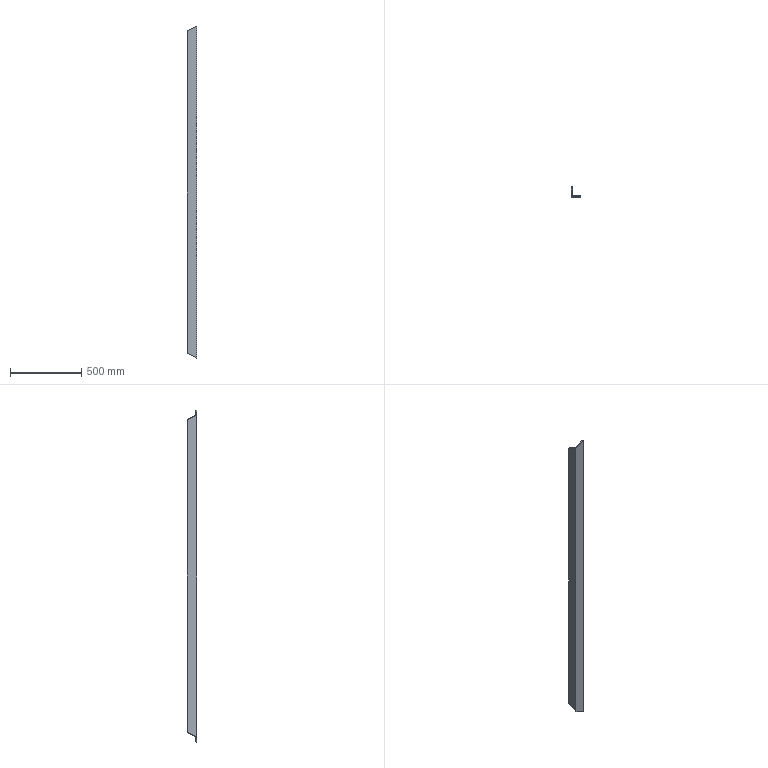Part | SolidWorks | features Extrusion 1, ICE 1 | 1 solid | 11 faces | box 70 x 70 x 2334 mm | volume 2413861 mm3 | plane 8 | cylinder 3 | commonest cylinder face diameters 6 x2 16 x1
STEP:
#1=CARTESIAN_POINT('',(5.,70.,2267.159));
#2=VERTEX_POINT('',#1);
#3=CARTESIAN_POINT('',(0.,70.,2264.683));
#4=VERTEX_POINT('',#3);
#5=CARTESIAN_POINT('',(31.579,70.,2280.318));
#6=DIRECTION('',(-0.8962,0.,-0.4437));
#7=VECTOR('',#6,1000.);
#8=LINE('',#5,#7);
#9=EDGE_CURVE('',#2,#4,#8,.T.);
#10=ORIENTED_EDGE('',*,*,#9,.F.);
#11=CARTESIAN_POINT('',(5.,70.,66.841));
#12=VERTEX_POINT('',#11);
#13=CARTESIAN_POINT('',(5.,70.,2334.));
#14=DIRECTION('',(0.,0.,-1.));
#15=VECTOR('',#14,1000.);
#16=LINE('',#13,#15);
#17=EDGE_CURVE('',#2,#12,#16,.T.);
#18=ORIENTED_EDGE('',*,*,#17,.T.);
#19=CARTESIAN_POINT('',(0.,70.,69.317));
#20=VERTEX_POINT('',#19);
#21=CARTESIAN_POINT('',(-896.516,70.,513.202));
#22=DIRECTION('',(0.8962,0.,-0.4437));
#23=VECTOR('',#22,1000.);
#24=LINE('',#21,#23);
#25=EDGE_CURVE('',#20,#12,#24,.T.);
#26=ORIENTED_EDGE('',*,*,#25,.F.);
#27=CARTESIAN_POINT('',(0.,70.,2334.));
#28=DIRECTION('',(0.,0.,-1.));
#29=VECTOR('',#28,1000.);
#30=LINE('',#27,#29);
#31=EDGE_CURVE('',#4,#20,#30,.T.);
#32=ORIENTED_EDGE('',*,*,#31,.F.);
#33=EDGE_LOOP('',(#10,#18,#26,#32));
#34=FACE_OUTER_BOUND('',#33,.T.);
#35=CARTESIAN_POINT('',(5.,70.,2334.));
#36=DIRECTION('',(0.,-1.,0.));
#37=DIRECTION('',(0.,0.,-1.));
#38=AXIS2_PLACEMENT_3D('',#35,#36,#37);
#39=PLANE('',#38);
#40=ADVANCED_FACE('',(#34),#39,.F.);
#41=CARTESIAN_POINT('',(0.,0.,2299.341));
#42=VERTEX_POINT('',#41);
#43=CARTESIAN_POINT('',(0.,42.437,2278.33));
#44=DIRECTION('',(0.,-0.8962,0.4437));
#45=VECTOR('',#44,1000.);
#46=LINE('',#43,#45);
#47=EDGE_CURVE('',#4,#42,#46,.T.);
#48=ORIENTED_EDGE('',*,*,#47,.F.);
#49=ORIENTED_EDGE('',*,*,#31,.T.);
#50=CARTESIAN_POINT('',(0.,0.,34.659));
#51=VERTEX_POINT('',#50);
#52=CARTESIAN_POINT('',(0.,970.532,515.19));
#53=DIRECTION('',(0.,0.8962,0.4437));
#54=VECTOR('',#53,1000.);
#55=LINE('',#52,#54);
#56=EDGE_CURVE('',#51,#20,#55,.T.);
#57=ORIENTED_EDGE('',*,*,#56,.F.);
#58=CARTESIAN_POINT('',(0.,0.,2334.));
#59=DIRECTION('',(0.,0.,-1.));
#60=VECTOR('',#59,1000.);
#61=LINE('',#58,#60);
#62=EDGE_CURVE('',#42,#51,#61,.T.);
#63=ORIENTED_EDGE('',*,*,#62,.F.);
#64=EDGE_LOOP('',(#48,#49,#57,#63));
#65=FACE_OUTER_BOUND('',#64,.T.);
#66=CARTESIAN_POINT('',(0.,70.,2334.));
#67=DIRECTION('',(1.,0.,0.));
#68=DIRECTION('',(0.,0.,-1.));
#69=AXIS2_PLACEMENT_3D('',#66,#67,#68);
#70=PLANE('',#69);
#71=ADVANCED_FACE('',(#65),#70,.F.);
#72=CARTESIAN_POINT('',(70.,0.,2334.));
#73=VERTEX_POINT('',#72);
#74=CARTESIAN_POINT('',(13.782,0.,2306.165));
#75=DIRECTION('',(0.8962,0.,0.4437));
#76=VECTOR('',#75,1000.);
#77=LINE('',#74,#76);
#78=EDGE_CURVE('',#42,#73,#77,.T.);
#79=ORIENTED_EDGE('',*,*,#78,.F.);
#80=ORIENTED_EDGE('',*,*,#62,.T.);
#81=CARTESIAN_POINT('',(70.,0.,0.));
#82=VERTEX_POINT('',#81);
#83=CARTESIAN_POINT('',(-914.314,0.,487.355));
#84=DIRECTION('',(-0.8962,0.,0.4437));
#85=VECTOR('',#84,1000.);
#86=LINE('',#83,#85);
#87=EDGE_CURVE('',#82,#51,#86,.T.);
#88=ORIENTED_EDGE('',*,*,#87,.F.);
#89=CARTESIAN_POINT('',(70.,0.,2334.));
#90=DIRECTION('',(0.,0.,-1.));
#91=VECTOR('',#90,1000.);
#92=LINE('',#89,#91);
#93=EDGE_CURVE('',#73,#82,#92,.T.);
#94=ORIENTED_EDGE('',*,*,#93,.F.);
#95=EDGE_LOOP('',(#79,#80,#88,#94));
#96=FACE_OUTER_BOUND('',#95,.T.);
#97=CARTESIAN_POINT('',(0.,0.,2334.));
#98=DIRECTION('',(0.,1.,0.));
#99=DIRECTION('',(0.,0.,1.));
#100=AXIS2_PLACEMENT_3D('',#97,#98,#99);
#101=PLANE('',#100);
#102=ADVANCED_FACE('',(#96),#101,.F.);
#103=CARTESIAN_POINT('',(70.,5.,2331.524));
#104=VERTEX_POINT('',#103);
#105=CARTESIAN_POINT('',(70.,0.,2334.));
#106=DIRECTION('',(0.,0.8962,-0.4437));
#107=VECTOR('',#106,1000.);
#108=LINE('',#105,#107);
#109=EDGE_CURVE('',#73,#104,#108,.T.);
#110=ORIENTED_EDGE('',*,*,#109,.F.);
#111=ORIENTED_EDGE('',*,*,#93,.T.);
#112=CARTESIAN_POINT('',(70.,5.,2.476));
#113=VERTEX_POINT('',#112);
#114=CARTESIAN_POINT('',(70.,928.095,459.52));
#115=DIRECTION('',(0.,-0.8962,-0.4437));
#116=VECTOR('',#115,1000.);
#117=LINE('',#114,#116);
#118=EDGE_CURVE('',#113,#82,#117,.T.);
#119=ORIENTED_EDGE('',*,*,#118,.F.);
#120=CARTESIAN_POINT('',(70.,5.,2334.));
#121=DIRECTION('',(0.,0.,-1.));
#122=VECTOR('',#121,1000.);
#123=LINE('',#120,#122);
#124=EDGE_CURVE('',#104,#113,#123,.T.);
#125=ORIENTED_EDGE('',*,*,#124,.F.);
#126=EDGE_LOOP('',(#110,#111,#119,#125));
#127=FACE_OUTER_BOUND('',#126,.T.);
#128=CARTESIAN_POINT('',(70.,0.,2334.));
#129=DIRECTION('',(-1.,0.,0.));
#130=DIRECTION('',(0.,0.,1.));
#131=AXIS2_PLACEMENT_3D('',#128,#129,#130);
#132=PLANE('',#131);
#133=ADVANCED_FACE('',(#127),#132,.F.);
#134=CARTESIAN_POINT('',(67.,8.,2328.554));
#135=VERTEX_POINT('',#134);
#136=CARTESIAN_POINT('',(70.,5.,2331.524));
#137=CARTESIAN_POINT('',(70.,6.757,2330.654));
#138=CARTESIAN_POINT('',(68.757,8.,2329.424));
#139=CARTESIAN_POINT('',(67.,8.,2328.554));
#140=(BOUNDED_CURVE()B_SPLINE_CURVE(3,(#136,#137,#138,#139),.UNSPECIFIED.,.F.,.F.)B_SPLINE_CURVE_WITH_KNOTS((4,4),(3.927,5.498),.UNSPECIFIED.)CURVE()GEOMETRIC_REPRESENTATION_ITEM()RATIONAL_B_SPLINE_CURVE((1.,0.8047,0.8047,1.))REPRESENTATION_ITEM(''));
#141=EDGE_CURVE('',#104,#135,#140,.T.);
#142=ORIENTED_EDGE('',*,*,#141,.F.);
#143=ORIENTED_EDGE('',*,*,#124,.T.);
#144=CARTESIAN_POINT('',(67.,8.,5.446));
#145=VERTEX_POINT('',#144);
#146=CARTESIAN_POINT('',(67.,8.,5.446));
#147=CARTESIAN_POINT('',(68.757,8.,4.576));
#148=CARTESIAN_POINT('',(70.,6.757,3.346));
#149=CARTESIAN_POINT('',(70.,5.,2.476));
#150=(BOUNDED_CURVE()B_SPLINE_CURVE(3,(#146,#147,#148,#149),.UNSPECIFIED.,.F.,.F.)B_SPLINE_CURVE_WITH_KNOTS((4,4),(3.927,5.498),.UNSPECIFIED.)CURVE()GEOMETRIC_REPRESENTATION_ITEM()RATIONAL_B_SPLINE_CURVE((1.,0.8047,0.8047,1.))REPRESENTATION_ITEM(''));
#151=EDGE_CURVE('',#145,#113,#150,.T.);
#152=ORIENTED_EDGE('',*,*,#151,.F.);
#153=CARTESIAN_POINT('',(67.,8.,2334.));
#154=DIRECTION('',(0.,0.,-1.));
#155=VECTOR('',#154,1000.);
#156=LINE('',#153,#155);
#157=EDGE_CURVE('',#135,#145,#156,.T.);
#158=ORIENTED_EDGE('',*,*,#157,.F.);
#159=EDGE_LOOP('',(#142,#143,#152,#158));
#160=FACE_OUTER_BOUND('',#159,.T.);
#161=CARTESIAN_POINT('',(67.,5.,2334.));
#162=DIRECTION('',(0.,0.,-1.));
#163=DIRECTION('',(-1.,0.,0.));
#164=AXIS2_PLACEMENT_3D('',#161,#162,#163);
#165=CYLINDRICAL_SURFACE('',#164,3.);
#166=ADVANCED_FACE('',(#160),#165,.T.);
#167=CARTESIAN_POINT('',(16.,8.,2303.302));
#168=VERTEX_POINT('',#167);
#169=CARTESIAN_POINT('',(69.166,8.,2329.626));
#170=DIRECTION('',(-0.8962,0.,-0.4437));
#171=VECTOR('',#170,1000.);
#172=LINE('',#169,#171);
#173=EDGE_CURVE('',#135,#168,#172,.T.);
#174=ORIENTED_EDGE('',*,*,#173,.F.);
#175=ORIENTED_EDGE('',*,*,#157,.T.);
#176=CARTESIAN_POINT('',(16.,8.,30.698));
#177=VERTEX_POINT('',#176);
#178=CARTESIAN_POINT('',(-858.93,8.,463.894));
#179=DIRECTION('',(0.8962,0.,-0.4437));
#180=VECTOR('',#179,1000.);
#181=LINE('',#178,#180);
#182=EDGE_CURVE('',#177,#145,#181,.T.);
#183=ORIENTED_EDGE('',*,*,#182,.F.);
#184=CARTESIAN_POINT('',(16.,8.,2334.));
#185=DIRECTION('',(0.,0.,-1.));
#186=VECTOR('',#185,1000.);
#187=LINE('',#184,#186);
#188=EDGE_CURVE('',#168,#177,#187,.T.);
#189=ORIENTED_EDGE('',*,*,#188,.F.);
#190=EDGE_LOOP('',(#174,#175,#183,#189));
#191=FACE_OUTER_BOUND('',#190,.T.);
#192=CARTESIAN_POINT('',(67.,8.,2334.));
#193=DIRECTION('',(0.,-1.,0.));
#194=DIRECTION('',(1.,0.,0.));
#195=AXIS2_PLACEMENT_3D('',#192,#193,#194);
#196=PLANE('',#195);
#197=ADVANCED_FACE('',(#191),#196,.F.);
#198=CARTESIAN_POINT('',(8.,16.,2295.381));
#199=VERTEX_POINT('',#198);
#200=CARTESIAN_POINT('',(16.,8.,2303.302));
#201=CARTESIAN_POINT('',(11.314,8.,2300.982));
#202=CARTESIAN_POINT('',(8.,11.314,2297.701));
#203=CARTESIAN_POINT('',(8.,16.,2295.381));
#204=(BOUNDED_CURVE()B_SPLINE_CURVE(3,(#200,#201,#202,#203),.UNSPECIFIED.,.F.,.F.)B_SPLINE_CURVE_WITH_KNOTS((4,4),(3.927,5.498),.UNSPECIFIED.)CURVE()GEOMETRIC_REPRESENTATION_ITEM()RATIONAL_B_SPLINE_CURVE((1.,0.8047,0.8047,1.))REPRESENTATION_ITEM(''));
#205=EDGE_CURVE('',#168,#199,#204,.T.);
#206=ORIENTED_EDGE('',*,*,#205,.F.);
#207=ORIENTED_EDGE('',*,*,#188,.T.);
#208=CARTESIAN_POINT('',(8.,16.,38.619));
#209=VERTEX_POINT('',#208);
#210=CARTESIAN_POINT('',(8.,16.,38.619));
#211=CARTESIAN_POINT('',(8.,11.314,36.299));
#212=CARTESIAN_POINT('',(11.314,8.,33.018));
#213=CARTESIAN_POINT('',(16.,8.,30.698));
#214=(BOUNDED_CURVE()B_SPLINE_CURVE(3,(#210,#211,#212,#213),.UNSPECIFIED.,.F.,.F.)B_SPLINE_CURVE_WITH_KNOTS((4,4),(3.927,5.498),.UNSPECIFIED.)CURVE()GEOMETRIC_REPRESENTATION_ITEM()RATIONAL_B_SPLINE_CURVE((1.,0.8047,0.8047,1.))REPRESENTATION_ITEM(''));
#215=EDGE_CURVE('',#209,#177,#214,.T.);
#216=ORIENTED_EDGE('',*,*,#215,.F.);
#217=CARTESIAN_POINT('',(8.,16.,2334.));
#218=DIRECTION('',(0.,0.,-1.));
#219=VECTOR('',#218,1000.);
#220=LINE('',#217,#219);
#221=EDGE_CURVE('',#199,#209,#220,.T.);
#222=ORIENTED_EDGE('',*,*,#221,.F.);
#223=EDGE_LOOP('',(#206,#207,#216,#222));
#224=FACE_OUTER_BOUND('',#223,.T.);
#225=CARTESIAN_POINT('',(16.,16.,2334.));
#226=DIRECTION('',(0.,0.,-1.));
#227=DIRECTION('',(-1.,0.,0.));
#228=AXIS2_PLACEMENT_3D('',#225,#226,#227);
#229=CYLINDRICAL_SURFACE('',#228,8.);
#230=ADVANCED_FACE('',(#224),#229,.F.);
#231=CARTESIAN_POINT('',(8.,67.,2270.129));
#232=VERTEX_POINT('',#231);
#233=CARTESIAN_POINT('',(8.,0.6433,2302.984));
#234=DIRECTION('',(0.,0.8962,-0.4437));
#235=VECTOR('',#234,1000.);
#236=LINE('',#233,#235);
#237=EDGE_CURVE('',#199,#232,#236,.T.);
#238=ORIENTED_EDGE('',*,*,#237,.F.);
#239=ORIENTED_EDGE('',*,*,#221,.T.);
#240=CARTESIAN_POINT('',(8.,67.,63.871));
#241=VERTEX_POINT('',#240);
#242=CARTESIAN_POINT('',(8.,928.739,490.536));
#243=DIRECTION('',(0.,-0.8962,-0.4437));
#244=VECTOR('',#243,1000.);
#245=LINE('',#242,#244);
#246=EDGE_CURVE('',#241,#209,#245,.T.);
#247=ORIENTED_EDGE('',*,*,#246,.F.);
#248=CARTESIAN_POINT('',(8.,67.,2334.));
#249=DIRECTION('',(0.,0.,-1.));
#250=VECTOR('',#249,1000.);
#251=LINE('',#248,#250);
#252=EDGE_CURVE('',#232,#241,#251,.T.);
#253=ORIENTED_EDGE('',*,*,#252,.F.);
#254=EDGE_LOOP('',(#238,#239,#247,#253));
#255=FACE_OUTER_BOUND('',#254,.T.);
#256=CARTESIAN_POINT('',(8.,16.,2334.));
#257=DIRECTION('',(-1.,0.,0.));
#258=DIRECTION('',(0.,-1.,0.));
#259=AXIS2_PLACEMENT_3D('',#256,#257,#258);
#260=PLANE('',#259);
#261=ADVANCED_FACE('',(#255),#260,.F.);
#262=CARTESIAN_POINT('',(8.,67.,2270.129));
#263=CARTESIAN_POINT('',(8.,68.757,2269.259));
#264=CARTESIAN_POINT('',(6.757,70.,2268.029));
#265=CARTESIAN_POINT('',(5.,70.,2267.159));
#266=(BOUNDED_CURVE()B_SPLINE_CURVE(3,(#262,#263,#264,#265),.UNSPECIFIED.,.F.,.F.)B_SPLINE_CURVE_WITH_KNOTS((4,4),(3.927,5.498),.UNSPECIFIED.)CURVE()GEOMETRIC_REPRESENTATION_ITEM()RATIONAL_B_SPLINE_CURVE((1.,0.8047,0.8047,1.))REPRESENTATION_ITEM(''));
#267=EDGE_CURVE('',#232,#2,#266,.T.);
#268=ORIENTED_EDGE('',*,*,#267,.F.);
#269=ORIENTED_EDGE('',*,*,#252,.T.);
#270=CARTESIAN_POINT('',(5.,70.,66.841));
#271=CARTESIAN_POINT('',(6.757,70.,65.971));
#272=CARTESIAN_POINT('',(8.,68.757,64.741));
#273=CARTESIAN_POINT('',(8.,67.,63.871));
#274=(BOUNDED_CURVE()B_SPLINE_CURVE(3,(#270,#271,#272,#273),.UNSPECIFIED.,.F.,.F.)B_SPLINE_CURVE_WITH_KNOTS((4,4),(3.927,5.498),.UNSPECIFIED.)CURVE()GEOMETRIC_REPRESENTATION_ITEM()RATIONAL_B_SPLINE_CURVE((1.,0.8047,0.8047,1.))REPRESENTATION_ITEM(''));
#275=EDGE_CURVE('',#12,#241,#274,.T.);
#276=ORIENTED_EDGE('',*,*,#275,.F.);
#277=ORIENTED_EDGE('',*,*,#17,.F.);
#278=EDGE_LOOP('',(#268,#269,#276,#277));
#279=FACE_OUTER_BOUND('',#278,.T.);
#280=CARTESIAN_POINT('',(5.,67.,2334.));
#281=DIRECTION('',(0.,0.,-1.));
#282=DIRECTION('',(-1.,0.,0.));
#283=AXIS2_PLACEMENT_3D('',#280,#281,#282);
#284=CYLINDRICAL_SURFACE('',#283,3.);
#285=ADVANCED_FACE('',(#279),#284,.T.);
#286=ORIENTED_EDGE('',*,*,#25,.T.);
#287=ORIENTED_EDGE('',*,*,#275,.T.);
#288=ORIENTED_EDGE('',*,*,#246,.T.);
#289=ORIENTED_EDGE('',*,*,#215,.T.);
#290=ORIENTED_EDGE('',*,*,#182,.T.);
#291=ORIENTED_EDGE('',*,*,#151,.T.);
#292=ORIENTED_EDGE('',*,*,#118,.T.);
#293=ORIENTED_EDGE('',*,*,#87,.T.);
#294=ORIENTED_EDGE('',*,*,#56,.T.);
#295=EDGE_LOOP('',(#286,#287,#288,#289,#290,#291,#292,#293,#294));
#296=FACE_OUTER_BOUND('',#295,.T.);
#297=CARTESIAN_POINT('',(105.,35.,0.));
#298=DIRECTION('',(-0.4056,0.4056,-0.8192));
#299=DIRECTION('',(0.,0.8962,0.4437));
#300=AXIS2_PLACEMENT_3D('',#297,#298,#299);
#301=PLANE('',#300);
#302=ADVANCED_FACE('',(#296),#301,.T.);
#303=ORIENTED_EDGE('',*,*,#9,.T.);
#304=ORIENTED_EDGE('',*,*,#47,.T.);
#305=ORIENTED_EDGE('',*,*,#78,.T.);
#306=ORIENTED_EDGE('',*,*,#109,.T.);
#307=ORIENTED_EDGE('',*,*,#141,.T.);
#308=ORIENTED_EDGE('',*,*,#173,.T.);
#309=ORIENTED_EDGE('',*,*,#205,.T.);
#310=ORIENTED_EDGE('',*,*,#237,.T.);
#311=ORIENTED_EDGE('',*,*,#267,.T.);
#312=EDGE_LOOP('',(#303,#304,#305,#306,#307,#308,#309,#310,#311));
#313=FACE_OUTER_BOUND('',#312,.T.);
#314=CARTESIAN_POINT('',(35.,105.,2264.683));
#315=DIRECTION('',(-0.4056,0.4056,0.8192));
#316=DIRECTION('',(0.,-0.8962,0.4437));
#317=AXIS2_PLACEMENT_3D('',#314,#315,#316);
#318=PLANE('',#317);
#319=ADVANCED_FACE('',(#313),#318,.T.);
#320=CLOSED_SHELL('',(#40,#71,#102,#133,#166,#197,#230,#261,#285,#302,#319));
#321=MANIFOLD_SOLID_BREP('',#320);
#322=CARTESIAN_POINT('',(0.,0.,0.));
#323=DIRECTION('',(0.,0.,1.));
#324=DIRECTION('',(1.,0.,0.));
#325=AXIS2_PLACEMENT_3D('',#322,#323,#324);
#326=(LENGTH_UNIT()NAMED_UNIT(*)SI_UNIT(.MILLI.,.METRE.));
#327=UNCERTAINTY_MEASURE_WITH_UNIT(LENGTH_MEASURE(0.00001),#326,'','');
#328=(NAMED_UNIT(*)PLANE_ANGLE_UNIT()SI_UNIT($,.RADIAN.));
#329=(NAMED_UNIT(*)SI_UNIT($,.STERADIAN.)SOLID_ANGLE_UNIT());
#330=(GEOMETRIC_REPRESENTATION_CONTEXT(3)GLOBAL_UNCERTAINTY_ASSIGNED_CONTEXT((#327))GLOBAL_UNIT_ASSIGNED_CONTEXT((#326,#328,#329))REPRESENTATION_CONTEXT('',''));
#331=ADVANCED_BREP_SHAPE_REPRESENTATION('',(#321,#325),#330);